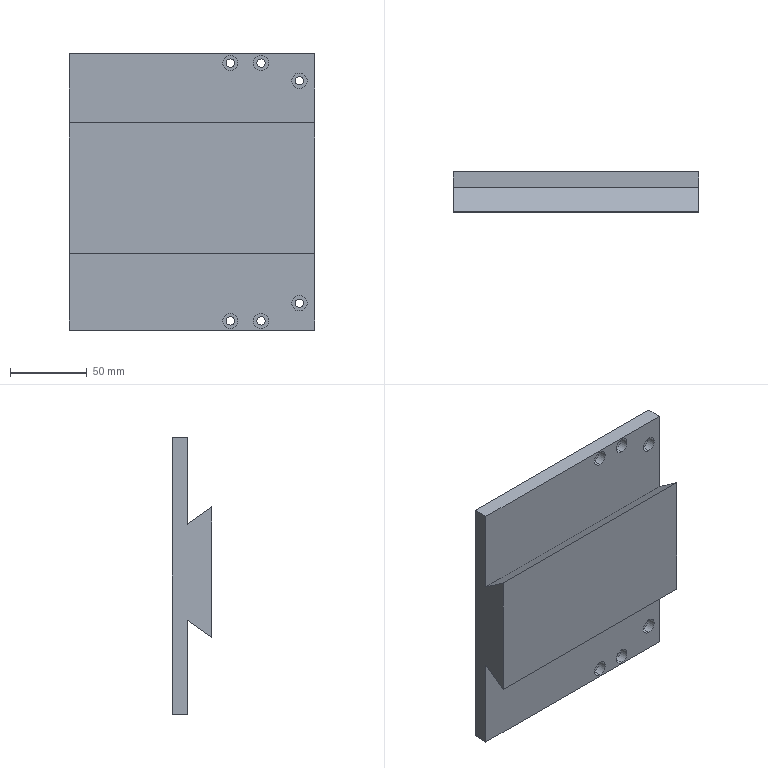Part | STEP file | 06-33 Front-rear adjusting dovetail plate | 1 solid | 40 faces | box 160 x 26 x 180 mm | volume 473686 mm3 | cylinder 24 | plane 16 | commonest cylinder face diameters 5.5 x12 10 x12